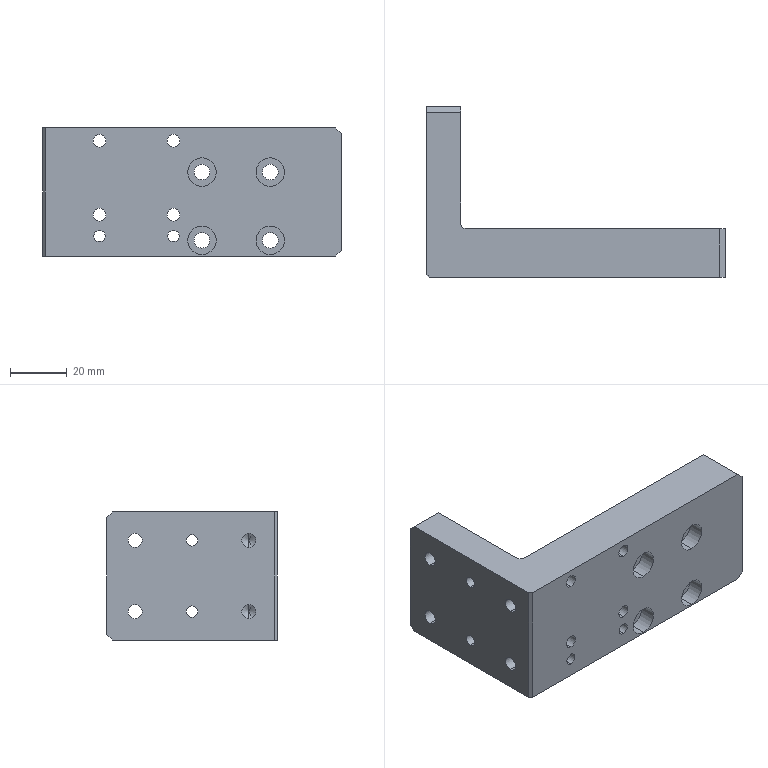Part | SolidWorks | features HoleWzd 6, Chamfer 2, Extrusion 1, Fillet 1 | 1 solid | 70 faces | box 105 x 60 x 45 mm | volume 97512 mm3 | cylinder 45 | plane 17 | cone 8 | commonest cylinder face diameters 4 x9 4.5 x8 5 x8 5.5 x8 10 x8 3.3 x4